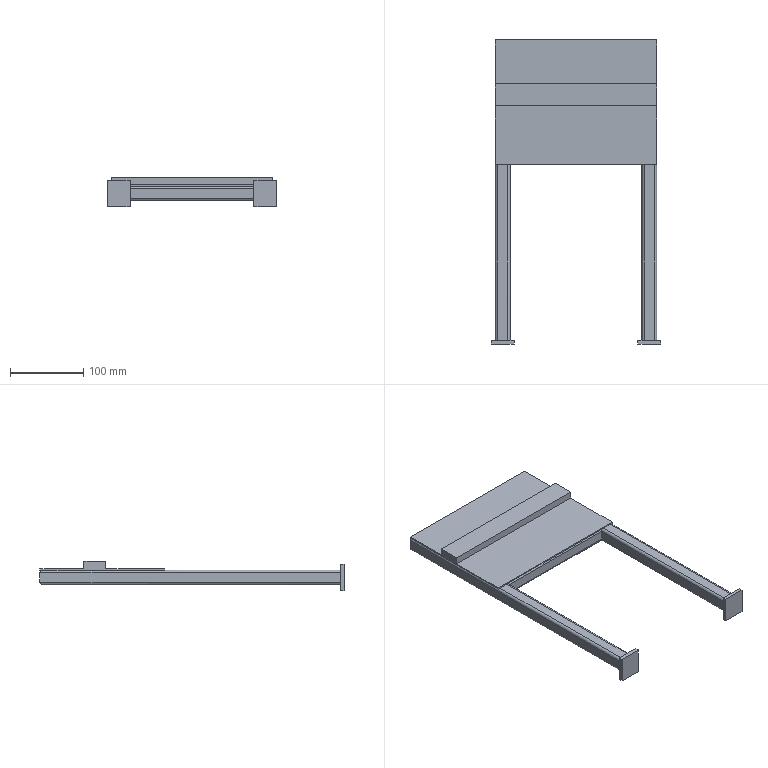Part | SolidWorks | features ICE 3, WeldMemberFeat 1, WeldmentFeature 1 | 1 solid | 112 faces | box 231.174 x 415 x 40.019 mm | volume 315048 mm3 | plane 72 | cylinder 40 | commonest cylinder face diameters 3.5 x20 7 x20